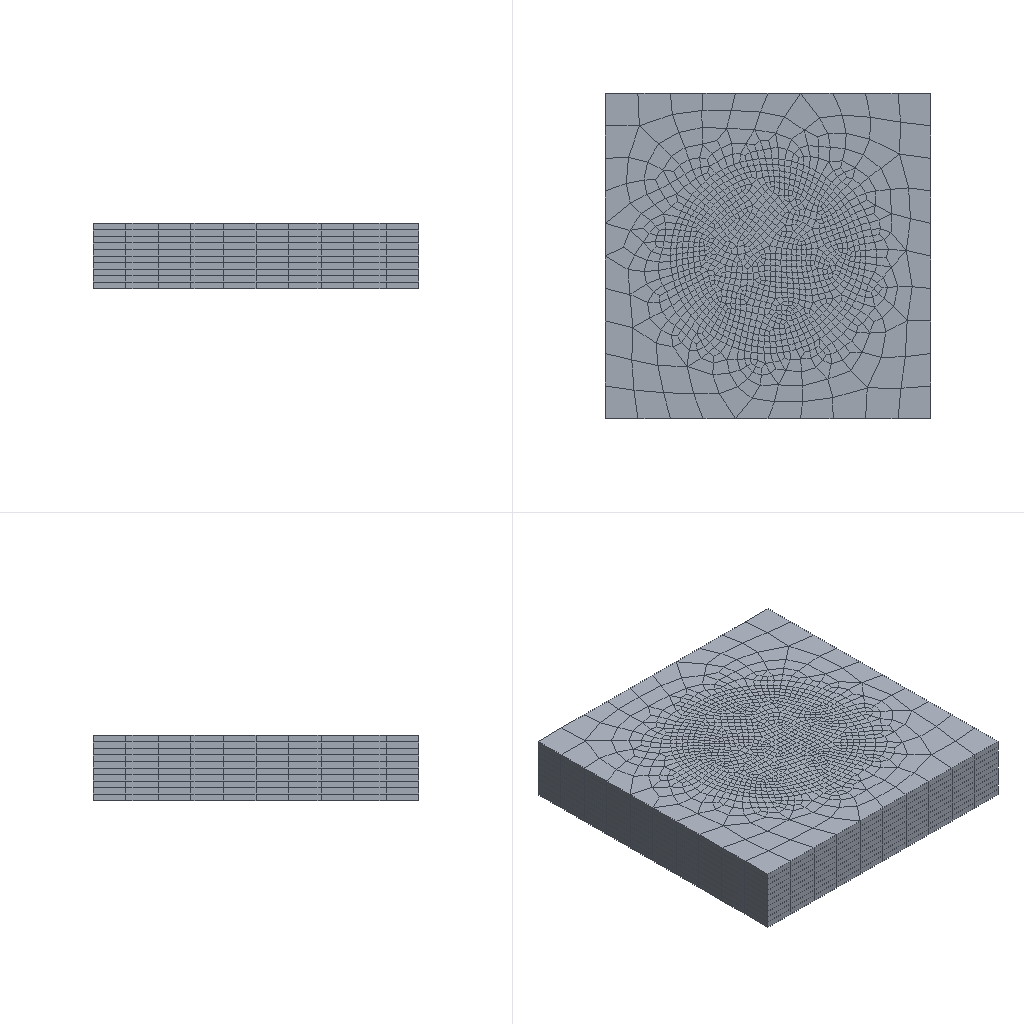Simulation study | abaqus
Set-up summary:
category,name,step,type,value,unit,region
solver,abaqus
solver,version,,,Abaqus/Explicit 2020
units,not stated in the deck,,not stated
analysis,deck,,transient,transient
load_step,Step-1,Step-1,transient
load_step,requested,,,1
mesh,nodes,,,18472
mesh,elements,,,16936
element_type,R3D3,,rigid,84
element_type,R3D4,,rigid,3372
element_type,C3D8R,,solid,13480
load,load commands in deck,,count,2
bc,support commands in deck,,count,7
material,MATERIAL-1,,in results
check,setup vs results,,match,"per instance, exact: element labels, types and connectivity; labels of the nodes the elements use; coordinates of those nodes at SINGLE_PRECISION in 2 of 2 instance(s)"
Abaqus input file, long lists of numbers shortened:
*Heading
** Job name: Job-2 Model name: Model-1
** Generated by: Abaqus/CAE 2020
*Preprint, echo=NO, model=NO, history=NO, contact=NO
**
** PARTS
**
*Part, name=work
*Node
      1,           0.,           0.,           0.
      2,          50.,           0.,           0.
** (15057 more lines like these left out)
*Element, type=C3D8R
   1,  578,  313,  324,  401, 4218, 3953, 3964, 4041
   2,  425,  455,  401,  324, 4065, 4095, 4041, 3964
** (13478 more lines like these left out)
*Nset, nset=Set-5, generate
     1,  15059,      1
*Elset, elset=Set-5, generate
     1,  13480,      1
** Section: Section-1
*Solid Section, elset=Set-5, material=Material-1
,
*End Part
**
*Part, name=zuantou
*Node
      1,   4.8,           0.,   19.492
      2,   4.8,           0.,   18.441
** (3410 more lines like these left out)
*Element, type=R3D4
1, 1, 2, 3, 4
2, 5, 6, 7, 8
** (3370 more lines like these left out)
*Element, type=R3D3
437, 858, 856,   7
438, 965, 951, 964
** (82 more lines like these left out)
*Node
   3413,           0., 4.4408921e-16,   21.455
*Nset, nset=zuantou-RefPt_, internal
3413,
*Elset, elset=zuantou, generate
    1,  3456,     1
*End Part
**
**
** ASSEMBLY
**
*Assembly, name=Assembly
**
*Instance, name=work-1, part=work
*End Instance
**
*Instance, name=zuantou-1, part=zuantou
         25.,         -25.,    -20.055
*End Instance
**
*Nset, nset=Set-2, instance=zuantou-1
 3413,
*Nset, nset=Set-3, instance=work-1
    1,    2,    3,    4,    6,    7,    8,    9,   11,   12,   13,   14,   15,   16,   17,   18
   19,   20,   21,   22,   23,   24,   25,   26,   27,   28,   29,   30,   31,   32,   33,   34
** (26 more lines like these left out)
*Elset, elset=Set-3, instance=work-1
   24,   32,   40,   48,  263,  281,  284,  293,  295,  297,  298,  302,  304,  305,  306,  307
  308,  312,  315,  316,  317,  318,  320,  323,  327,  328,  329,  330,  331,  332,  334,  335
** (21 more lines like these left out)
*Nset, nset=s_Set-1, instance=work-1
     5,    10,    47,    48,    49,    50,    51,    52,    53,    54,    55,    56,    57,    58,    59,    60
    61,    62,    63,    64,    65,    66,    67,    68,    69,    70,    71,    72,    73,    74,    75,    76
** (706 more lines like these left out)
*Elset, elset=s_Set-1, instance=work-1, generate
  3671,  13480,      1
*Elset, elset=_m_Surf-1_SPOS, internal, instance=zuantou-1, generate
    1,  3456,     1
*Surface, type=ELEMENT, name=m_Surf-1
_m_Surf-1_SPOS, SPOS
*Surface, type=NODE, name=s_Set-1_CNS_, internal
s_Set-1, 1.
*Rigid Body, ref node=zuantou-1.zuantou-RefPt_, elset=zuantou-1.zuantou
*End Assembly
**
** MATERIALS
**
*Material, name=Material-1
*Damage Initiation, criterion=SHEAR
 0.5,0.,0.
*Damage Evolution, type=DISPLACEMENT
 0.0001,
*Density
 8.28e-09,
*Elastic
210000., 0.3
*Plastic
350.,   0.
389., 0.05
**
** INTERACTION PROPERTIES
**
*Surface Interaction, name=IntProp-1
*Friction
 0.15,
*Surface Behavior, pressure-overclosure=HARD
** ----------------------------------------------------------------
**
** STEP: Step-1
**
*Step, name=Step-1, nlgeom=YES
*Dynamic, Explicit
, 0.1
*Bulk Viscosity
0.06, 1.2
** Mass Scaling: Semi-Automatic
**               Whole Model
*Fixed Mass Scaling, factor=500.
**
** BOUNDARY CONDITIONS
**
** Name: BC-1 Type: 速度/角速度
*Boundary, type=VELOCITY
Set-2, 1, 1
Set-2, 2, 2
Set-2, 3, 3, 110.
Set-2, 4, 4
Set-2, 5, 5
Set-2, 6, 6, 314.
** Name: BC-2 Type: 对称/反对称/完全固定
*Boundary
Set-3, ENCASTRE
**
** INTERACTIONS
**
** Interaction: Int-1
*Contact Pair, interaction=IntProp-1, mechanical constraint=KINEMATIC, cpset=Int-1
m_Surf-1, s_Set-1_CNS_
**
** OUTPUT REQUESTS
**
*Restart, write, number interval=1, time marks=NO
**
** FIELD OUTPUT: F-Output-1
**
*Output, field, number interval=50
*Node Output
A, RF, RM, RT, U, V
*Element Output, directions=YES
E, EVF, LE, MISES, MISESMAX, PE, PEEQ, PEEQMAX, PEEQT, PEEQVAVG, PEMAG, PEVAVG, S, STATUS, SVAVG
*Contact Output
CDISP, CSTRESS
**
** HISTORY OUTPUT: H-Output-1
**
*Output, history, time interval=1e-06
*Node Output, nset=Set-2
RF1, RF2, RF3
*End Step
Results summary:
result,step,Step-1,completed,increments=45542 time=0.1/0.1
result,analysis,,,transient
result,last_loadstep,,,1
result,primary field,,,U
result,reaction total,,FX,-10871.726,model units
result,reaction total,,FY,-11279.85,model units
result,reaction total,,FZ,-3867.774,model units